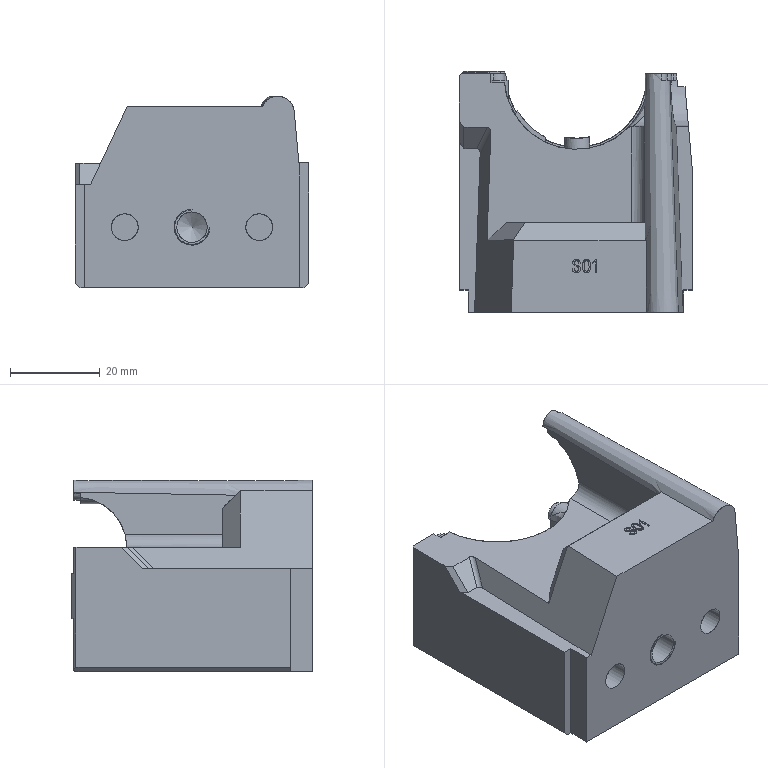NC program | PowerMill | posted with a generic post | part box 52 x 53.756 x 42.711 mm
Lines 1 to 783 of 10927:
%
O0001
N104 ( POWERMILL CB  : 2026004.0)
N105 ( POST VER      : 2026.0.0.5161)
N106 ( OPTION FILE   : FANUC)
N107 ( OUTPUT WORKPLANE : 2)
N108 (  )
N109 ( TOOL LIST )
N110 (------------------------------------)
N111 ( NO. | ID     | DIA.| TIP RAD|LENGTH)
N112 (------------------------------------)
N113 (    1|R3_1_1_1| 6.0 |  3.0   |109.48)
N114 (------------------------------------)
N115 (  )
N116 ( NUMBER OF TOOLPATHS: 2.0 )
N117 ( ESTIMATED PROGRAM DURATION: 0 HOURS 1 MIN 5 SEC)
N118 (  )
N119 G00 G21 G80 G40 G17
N120 G90
N121 G54
N122 G53 Z0.0
N123 (---------------)
N124 ( START TOOLPATH : 09中光-R3-平行-已选面 )
N125 (---------------)
N126 ( TOOL NO.    :1 )
N127 ( TOOL TYPE   : BALLNOSED)
N128 ( TOOL ID     : R3_1_1_1)
N129 ( TOOL DIA    : 6.0 LENGTH 109.48)
N130 T1
N131 M6
N132 S5500 M03
N133 G00 G90 X10.1509 Y13.0999
N134 G43 Z75.756 H1
N135
N136 G05 P10000 R8
N137 Z46.1775
N138 G01 Z43.1775 F2400.0
N139 X9.8219 Y12.7709 Z42.643 F4000.0
N140 X9.7601 Y12.7091 Z42.5428
N141 X9.7378 Y12.6936 Z42.5082
N142 X9.7126 Y12.6885 Z42.4726
N143 X9.6347 Y12.6893 Z42.3666
N144 X9.6137 Y12.7039 Z42.3403
N145 X9.6039 Y12.7473 Z42.3337
N146 X9.615 Y12.7761 Z42.3535
N147 X10.0693 Y13.2304 Z43.0441
N148 X10.3226 Y13.4837 Z43.4582
N149 X10.4866 Y13.6477 Z43.7076
N150 X10.5177 Y13.6788 Z43.7548
N151 X10.5392 Y13.7133 Z43.7877
N152 X10.5506 Y13.7612 Z43.8053
N153 X10.5572 Y13.8242 Z43.816
N154 X10.5535 Y13.8633 Z43.8107
N155 X10.5331 Y13.8905 Z43.7799
N156 X10.5116 Y13.8848 Z43.7471
N157 X10.3132 Y13.6865 Z43.4429
N158 X9.9632 Y13.3364 Z42.8782
N159 X9.4112 Y12.7844 Z42.0845
N160 X9.3531 Y12.7263 Z42.001
N161 X9.329 Y12.7098 Z41.9681
N162 X9.3018 Y12.7048 Z41.9339
N163 X9.2282 Y12.707 Z41.8449
N164 X9.2061 Y12.7217 Z41.82
N165 X9.1963 Y12.7642 Z41.8133
N166 X9.2081 Y12.7935 Z41.8313
N167 X9.6577 Y13.2431 Z42.4319
N168 X9.9859 Y13.5713 Z42.9114
N169 X10.3787 Y13.9641 Z43.5499
N170 X10.5156 Y14.101 Z43.7453
N171 X10.5378 Y14.1231 Z43.777
N172 X10.56 Y14.1619 Z43.8089
N173 X10.568 Y14.2149 Z43.8207
N174 X10.5678 Y14.259 Z43.8209
N175 X10.5601 Y14.297 Z43.8102
N176 X10.5376 Y14.3199 Z43.778
N177 X10.5151 Y14.3126 Z43.7455
N178 X10.3659 Y14.1634 Z43.5291
N179 X9.9776 Y13.7751 Z42.8993
N180 X9.6552 Y13.4527 Z42.4286
N181 X9.4 Y13.1975 Z42.0938
N182 X9.0072 Y12.8047 Z41.5949
N183 X8.9517 Y12.7492 Z41.5245
N184 X8.926 Y12.7317 Z41.4931
N185 X8.8968 Y12.7265 Z41.4603
N186 X8.8264 Y12.7296 Z41.3833
N187 X8.8035 Y12.7443 Z41.3599
N188 X8.7935 Y12.7859 Z41.3534
N189 X8.8057 Y12.8153 Z41.3699
N190 X9.322 Y13.3317 Z41.9916
N191 X9.6928 Y13.7024 Z42.4831
N192 X10.042 Y14.0516 Z42.9994
N193 X10.4706 Y14.4803 Z43.6898
N194 X10.5147 Y14.5243 Z43.7459
N195 X10.5396 Y14.5492 Z43.7776
N196 X10.562 Y14.5875 Z43.8068
N197 X10.5695 Y14.6388 Z43.8182
N198 X10.5689 Y14.6829 Z43.8192
N199 X10.5607 Y14.7209 Z43.8093
N200 X10.5376 Y14.7439 Z43.7777
N201 X10.5149 Y14.7367 Z43.7454
N202 X10.364 Y14.5858 Z43.526
N203 X9.9783 Y14.2001 Z42.9003
N204 X9.6517 Y13.8735 Z42.424
N205 X9.3429 Y13.5646 Z42.0189
N206 X8.9741 Y13.1959 Z41.5757
N207 X8.6042 Y12.8259 Z41.1544
N208 X8.5461 Y12.7679 Z41.0882
N209 X8.5193 Y12.7492 Z41.0588
N210 X8.489 Y12.7428 Z41.0276
N211 X8.4151 Y12.7426 Z40.9537
N212 X8.3912 Y12.7562 Z40.931
N213 X8.3805 Y12.7972 Z40.9238
N214 X8.3931 Y12.827 Z40.9388
N215 X8.8948 Y13.3287 Z41.482
N216 X9.265 Y13.6989 Z41.9192
N217 X9.7006 Y14.1344 Z42.4944
N218 X9.9965 Y14.4304 Z42.9268
N219 X10.3955 Y14.8294 Z43.5767
N220 X10.5158 Y14.9497 Z43.7447
N221 X10.5384 Y14.9723 Z43.7763
N222 X10.5603 Y15.0106 Z43.8075
N223 X10.5677 Y15.0628 Z43.8195
N224 X10.567 Y15.1062 Z43.8202
N225 X10.5589 Y15.1441 Z43.8101
N226 X10.5363 Y15.1671 Z43.7782
N227 X10.514 Y15.16 Z43.7458
N228 X10.3469 Y14.9929 Z43.498
N229 X10.0228 Y14.6688 Z42.9681
N230 X9.673 Y14.319 Z42.4542
N231 X9.2368 Y13.8828 Z41.8859
N232 X8.8781 Y13.5241 Z41.4629
N233 X8.5594 Y13.2054 Z41.1234
N234 X8.1745 Y12.8205 Z40.7278
N235 X8.1125 Y12.7585 Z40.664
N236 X8.0849 Y12.7389 Z40.6367
N237 X8.0538 Y12.7309 Z40.6073
N238 X7.9746 Y12.7265 Z40.5346
N239 X7.9498 Y12.7387 Z40.5126
N240 X7.9383 Y12.7791 Z40.5047
N241 X7.951 Y12.8091 Z40.5183
N242 X8.4532 Y13.3114 Z41.0111
N243 X8.914 Y13.7722 Z41.5047
N244 X9.2658 Y14.124 Z41.9201
N245 X9.7024 Y14.5606 Z42.4972
N246 X9.9981 Y14.8562 Z42.9292
N247 X10.3995 Y15.2577 Z43.583
N248 X10.4961 Y15.3543 Z43.7173
N249 X10.5025 Y15.3607 Z43.7262
N250 X10.5261 Y15.4106 Z43.7596
N251 X10.5243 Y15.4752 Z43.7589
N252 X10.5219 Y15.4847 Z43.7559
N253 X10.4934 Y15.5314 Z43.7166
N254 X10.4558 Y15.5261 Z43.6609
N255 X10.3202 Y15.3904 Z43.4542
N256 X10.0476 Y15.1179 Z43.0085
N257 X9.6376 Y14.7079 Z42.4056
N258 X9.2961 Y14.3664 Z41.9575
N259 X8.8542 Y13.9245 Z41.4374
N260 X8.4226 Y13.4929 Z40.9817
N261 X7.7332 Y12.8035 Z40.329
N262 X7.6801 Y12.7504 Z40.2787
N263 X7.6512 Y12.7307 Z40.2523
N264 X7.6185 Y12.7243 Z40.2241
N265 X7.5496 Y12.7257 Z40.1662
N266 X7.5246 Y12.7393 Z40.1463
N267 X7.5134 Y12.7789 Z40.1399
N268 X7.526 Y12.8085 Z40.1529
N269 X7.7741 Y13.0565 Z40.3808
N270 X8.0124 Y13.2949 Z40.5876
N271 X8.5224 Y13.8048 Z41.084
N272 X8.8797 Y14.1622 Z41.4646
N273 X9.2388 Y14.5212 Z41.8882
N274 X9.6759 Y14.9583 Z42.4583
N275 X10.0244 Y15.3069 Z42.9707
N276 X10.3754 Y15.6578 Z43.5403
N277 X10.3944 Y15.7105 Z43.5716
N278 X10.3823 Y15.7707 Z43.553
N279 X10.3704 Y15.7908 Z43.5343
N280 X10.3416 Y15.8158 Z43.4883
N281 X10.3106 Y15.8052 Z43.4384
N282 X10.2967 Y15.7913 Z43.4159
N283 X9.9756 Y15.4702 Z42.8964
N284 X9.6502 Y15.1448 Z42.4221
N285 X9.3327 Y14.8272 Z42.0055
N286 X8.87 Y14.3646 Z41.4543
N287 X8.5113 Y14.0059 Z41.0723
N288 X8.0059 Y13.5005 Z40.5819
N289 X7.3235 Y12.8181 Z39.9955
N290 X7.2728 Y12.7673 Z39.9518
N291 X7.243 Y12.7472 Z39.9272
N292 X7.209 Y12.7409 Z39.9006
N293 X7.1427 Y12.743 Z39.8502
N294 X7.1171 Y12.7567 Z39.8315
N295 X7.1058 Y12.7957 Z39.8252
N296 X7.1188 Y12.8255 Z39.8368
N297 X7.6223 Y13.329 Z40.2492
N298 X8.0103 Y13.717 Z40.5857
N299 X8.5202 Y14.2269 Z41.0817
N300 X8.878 Y14.5847 Z41.4628
N301 X9.2366 Y14.9433 Z41.8856
N302 X9.6727 Y15.3793 Z42.4537
N303 X10.0226 Y15.7293 Z42.9678
N304 X10.2167 Y15.9234 Z43.2851
N305 X10.2356 Y15.9764 Z43.316
N306 X10.2232 Y16.0359 Z43.2957
N307 X10.2098 Y16.0575 Z43.2738
N308 X10.1815 Y16.0809 Z43.2274
N309 X10.1511 Y16.0699 Z43.1778
N310 X10.1356 Y16.0544 Z43.1525
N311 X10.0426 Y15.9614 Z43.0004
N312 X9.6274 Y15.5462 Z42.3921
N313 X9.2788 Y15.1976 Z41.9354
N314 X8.9034 Y14.8222 Z41.4921
N315 X8.4994 Y14.4182 Z41.0595
N316 X8.0692 Y13.988 Z40.6419
N317 X7.6151 Y13.534 Z40.243
N318 X6.8996 Y12.8184 Z39.6753
N319 X6.8394 Y12.7582 Z39.6276
N320 X6.8101 Y12.7374 Z39.6051
N321 X6.7766 Y12.7283 Z39.5808
N322 X6.6971 Y12.722 Z39.5245
N323 X6.6705 Y12.7329 Z39.5069
N324 X6.657 Y12.7708 Z39.5009
N325 X6.6691 Y12.8001 Z39.5122
N326 X6.8177 Y12.9486 Z39.6302
N327 X7.0857 Y13.2166 Z39.8236
N328 X7.6226 Y13.7536 Z40.2495
N329 X8.0832 Y14.2142 Z40.6554
N330 X8.5251 Y14.656 Z41.0869
N331 X8.9493 Y15.0802 Z41.5463
N332 X9.2425 Y15.3734 Z41.8925
N333 X9.6509 Y15.7819 Z42.423
N334 X10.0501 Y16.181 Z43.0112
N335 X10.0665 Y16.2125 Z43.034
N336 X10.0692 Y16.2601 Z43.0335
N337 X10.0563 Y16.2927 Z43.0102
N338 X10.0367 Y16.3165 Z42.9772
N339 X10.007 Y16.333 Z42.9294
N340 X9.9752 Y16.3182 Z42.8823
N341 X9.9532 Y16.2963 Z42.8513
N342 X9.6846 Y16.0277 Z42.4717
N343 X9.2581 Y15.6012 Z41.911
N344 X8.9073 Y15.2504 Z41.4967
N345 X8.4379 Y14.781 Z40.9964
N346 X7.9733 Y14.3164 Z40.5536
N347 X7.571 Y13.9141 Z40.2047
N348 X7.1647 Y13.5078 Z39.8853
N349 X6.4391 Y12.7822 Z39.3593
N350 X6.3885 Y12.7316 Z39.3226
N351 X6.358 Y12.7109 Z39.3016
N352 X6.3228 Y12.7037 Z39.2791
N353 X6.2547 Z39.2373
N354 X6.2278 Y12.7161 Z39.2217
N355 X6.215 Y12.7535 Z39.2168
N356 X6.2276 Y12.7829 Z39.2268
N357 X7.0472 Y13.6024 Z39.7945
N358 X7.5603 Y14.1155 Z40.1955
N359 X7.981 Y14.5362 Z40.5603
N360 X8.454 Y15.0092 Z41.0118
N361 X8.9459 Y15.5012 Z41.5424
N362 X9.2847 Y15.8399 Z41.9426
N363 X9.8384 Y16.3936 Z42.6673
N364 X9.8541 Y16.4267 Z42.6854
N365 X9.8495 Y16.4743 Z42.672
N366 X9.8292 Y16.49 Z42.6403
N367 X9.7522 Y16.4892 Z42.5288
N368 X9.722 Y16.4816 Z42.4866
N369 X9.6928 Y16.4601 Z42.4488
N370 X9.6216 Y16.3889 Z42.3607
N371 X9.2893 Y16.0567 Z41.9498
N372 X8.9504 Y15.7178 Z41.5476
N373 X8.4568 Y15.2241 Z41.0145
N374 X7.9823 Y14.7496 Z40.5614
N375 X7.5526 Y14.32 Z40.1888
N376 X7.0373 Y13.8047 Z39.7876
N377 X6.6215 Y13.3889 Z39.4958
N378 X6.0225 Y12.7899 Z39.1007
N379 X5.9758 Y12.7431 Z39.0699
N380 X5.9443 Y12.7221 Z39.0501
N381 X5.9078 Y12.7157 Z39.0289
N382 X5.8446 Y12.7178 Z38.9933
N383 X5.8176 Y12.731 Z38.9789
N384 X5.8051 Y12.7681 Z38.9745
N385 X5.8179 Y12.7974 Z38.9838
N386 X6.5866 Y13.5661 Z39.4713
N387 X7.0382 Y14.0176 Z39.7882
N388 X7.5848 Y14.5643 Z40.2168
N389 X7.9785 Y14.958 Z40.5581
N390 X8.4487 Y15.4282 Z41.0067
N391 X8.9328 Y15.9123 Z41.5268
N392 X9.4003 Y16.3797 Z42.0696
N393 X9.4156 Y16.4123 Z42.0855
N394 X9.4092 Y16.4579 Z42.0724
N395 X9.3873 Y16.4723 Z42.0431
N396 X9.3089 Y16.4694 Z41.9439
N397 X9.2774 Y16.461 Z41.9053
N398 X9.2474 Y16.439 Z41.871
N399 X9.1777 Y16.3693 Z41.7945
N400 X8.9219 Y16.1135 Z41.5138
N401 X8.4442 Y15.6358 Z41.0024
N402 X8.0672 Y15.2588 Z40.64
N403 X7.5426 Y14.7342 Z40.1805
N404 X7.0328 Y14.2244 Z39.7844
N405 X6.6154 Y13.807 Z39.4916
N406 X6.0326 Y13.2242 Z39.1211
N407 X5.6368 Y12.8284 Z38.8873
N408 X5.6039 Y12.7955 Z38.8679
N409 X5.5689 Y12.7743 Z38.8472
N410 X5.5296 Y12.7735 Z38.8238
N411 X5.4859 Y12.7844 Z38.7979
N412 X5.4531 Y12.8202 Z38.7806
N413 X5.4653 Y12.869 Z38.7919
N414 X5.5248 Y12.9286 Z38.8332
N415 X6.0857 Y13.4895 Z39.1544
N416 X6.5171 Y13.9209 Z39.4253
N417 X7.0287 Y14.4325 Z39.7816
N418 X7.5338 Y14.9375 Z40.1736
N419 X8.0473 Y15.451 Z40.6209
N420 X8.4315 Y15.8352 Z40.9902
N421 X8.9538 Y16.3575 Z41.5307
N422 X8.9686 Y16.3896 Z41.5447
N423 X8.9605 Y16.4332 Z41.5325
N424 X8.9373 Y16.4468 Z41.5057
N425 X8.8593 Y16.4431 Z41.4193
N426 X8.8268 Y16.4345 Z41.3843
N427 X8.7966 Y16.4125 Z41.3533
N428 X8.7298 Y16.3457 Z41.2871
N429 X8.4233 Y16.0391 Z40.983
N430 X8.0405 Y15.6563 Z40.6143
N431 X7.5154 Y15.1313 Z40.1593
N432 X7.0819 Y14.6978 Z39.8207
N433 X6.6125 Y14.2284 Z39.4895
N434 X6.1132 Y13.7291 Z39.1717
N435 X5.409 Y13.0249 Z38.7721
N436 X5.3511 Y12.9669 Z38.7311
N437 X5.3504 Y12.9663 Z38.7306
N438 X5.305 Y12.9539 Z38.7018
N439 X5.2671 Y12.989 Z38.6823
N440 X5.2592 Y13.0074 Z38.6794
N441 X5.2532 Y13.0591 Z38.6793
N442 X5.2757 Y13.1037 Z38.6935
N443 X5.2896 Y13.1176 Z38.7014
N444 X6.1172 Y13.9452 Z39.1742
N445 X6.5385 Y14.3665 Z39.4387
N446 X7.0755 Y14.9035 Z39.8157
N447 X7.5073 Y15.3353 Z40.1529
N448 X7.9886 Y15.8166 Z40.5669
N449 X8.5106 Y16.3386 Z41.0565
N450 X8.5254 Y16.3703 Z41.0692
N451 X8.5171 Y16.4128 Z41.058
N452 X8.4934 Y16.4271 Z41.0331
N453 X8.4228 Y16.4276 Z40.9621
N454 X8.389 Y16.4201 Z40.929
N455 X8.3579 Y16.398 Z40.9
N456 X8.2987 Y16.3388 Z40.8468
N457 X8.0019 Y16.0421 Z40.5799
N458 X7.5564 Y15.5965 Z40.1921
N459 X7.0174 Y15.0576 Z39.7737
N460 X6.5738 Y14.614 Z39.4624
N461 X6.0921 Y14.1322 Z39.1584
N462 X5.4483 Y13.4884 Z38.7945
N463 X5.2407 Y13.2808 Z38.6665
N464 X5.196 Y13.2723 Z38.6382
N465 X5.1695 Y13.3154 Z38.6204
N466 X5.1663 Y13.3631 Z38.6173
N467 X5.1726 Y13.4102 Z38.6207
N468 X5.1962 Y13.4485 Z38.6359
N469 X5.2265 Y13.4788 Z38.6558
N470 X5.3734 Y13.6257 Z38.7521
N471 X6.0778 Y14.33 Z39.1494
N472 X6.549 Y14.8013 Z39.4453
N473 X7.1199 Y15.3722 Z39.8504
N474 X7.5246 Y15.7769 Z40.1665
N475 X8.0963 Y16.3486 Z40.6516
N476 X8.1116 Y16.3804 Z40.6629
N477 X8.1039 Y16.4224 Z40.6516
N478 X8.0801 Y16.4375 Z40.6275
N479 X8.0161 Y16.4409 Z40.5666
N480 X7.9799 Y16.4341 Z40.5337
N481 X7.9462 Y16.4106 Z40.5064
N482 X7.8926 Y16.357 Z40.4657
N483 X7.7739 Y16.2383 Z40.3759
N484 X7.5081 Y15.9725 Z40.1536
N485 X7.0637 Y15.5281 Z39.8064
N486 X6.5333 Y14.9977 Z39.4354
N487 X6.1127 Y14.5771 Z39.1713
N488 X5.2862 Y13.7506 Z38.6993
N489 X5.2169 Y13.6813 Z38.6504
N490 X5.2164 Y13.6808 Z38.65
N491 X5.1728 Y13.6739 Z38.6209
N492 X5.1473 Y13.7178 Z38.6059
N493 X5.1448 Y13.7696 Z38.6064
N494 X5.1514 Y13.8144 Z38.6118
N495 X5.1744 Y13.851 Z38.6262
N496 X5.2087 Y13.8852 Z38.6469
N497 X5.5126 Y14.1891 Z38.8304
N498 X6.0425 Y14.7191 Z39.1273
N499 X6.6364 Y15.313 Z39.5063
N500 X7.1258 Y15.8024 Z39.855
N501 X7.6854 Y16.362 Z40.287
N502 X7.7006 Y16.3939 Z40.2969
N503 X7.6914 Y16.435 Z40.2847
N504 X7.6663 Y16.4481 Z40.2614
N505 X7.594 Y16.4458 Z40.1984
N506 X7.5575 Y16.4366 Z40.168
N507 X7.5237 Y16.4124 Z40.1431
N508 X7.4642 Y16.3528 Z40.1023
N509 X7.3183 Y16.2069 Z40.0024
N510 X7.0813 Y15.9699 Z39.8202
N511 X6.5233 Y15.412 Z39.4292
N512 X6.0623 Y14.9509 Z39.1397
N513 X5.4275 Y14.3162 Z38.7829
N514 X5.2079 Y14.0966 Z38.6453
N515 X5.1804 Y14.0849 Z38.6278
N516 X5.1497 Y14.1017 Z38.6079
N517 X5.1396 Y14.1342 Z38.601
N518 X5.1399 Y14.1913 Z38.6004
N519 X5.1485 Y14.2363 Z38.6055
N520 X5.1721 Y14.2729 Z38.6206
N521 X5.2086 Y14.3094 Z38.6443
N522 X5.3871 Y14.4879 Z38.7601
N523 X6.0919 Y15.1927 Z39.1583
N524 X6.5735 Y15.6743 Z39.4622
N525 X7.2426 Y16.3434 Z39.9293
N526 X7.2574 Y16.3749 Z39.9382
N527 X7.2473 Y16.4149 Z39.927
N528 X7.2214 Y16.4277 Z39.9058
N529 X7.1507 Y16.4259 Z39.8507
N530 X7.1138 Y16.417 Z39.8232
N531 X7.0803 Y16.3933 Z39.8005
N532 X7.0235 Y16.3364 Z39.7644
N533 X6.8295 Y16.1425 Z39.6412
N534 X6.6431 Y15.956 Z39.511
N535 X6.0498 Y15.3627 Z39.1319
N536 X5.3458 Y14.6587 Z38.7358
N537 X5.2088 Y14.5218 Z38.6439
N538 X5.1815 Y14.5103 Z38.6256
N539 X5.1512 Y14.5274 Z38.6052
N540 X5.1411 Y14.5601 Z38.5984
N541 Y14.6164
N542 X5.1494 Y14.6614 Z38.604
N543 X5.1729 Y14.698 Z38.6198
N544 X5.2089 Y14.7339 Z38.6439
N545 X5.3459 Y14.871 Z38.7359
N546 X6.05 Y15.575 Z39.132
N547 X6.8271 Y16.3522 Z39.6255
N548 X6.8421 Y16.3834 Z39.6337
N549 X6.8331 Y16.4231 Z39.6238
N550 X6.8076 Y16.4382 Z39.6042
N551 X6.7496 Y16.4431 Z39.5621
N552 X6.7114 Y16.4372 Z39.5355
N553 X6.6768 Y16.414 Z39.5137
N554 X6.6306 Y16.3678 Z39.4865
N555 X6.381 Y16.1182 Z39.3397
N556 X6.0588 Y15.796 Z39.1375
N557 X5.3537 Y15.0909 Z38.7405
N558 X5.2089 Y14.9461 Z38.644
N559 X5.1816 Y14.9346 Z38.6257
N560 X5.1513 Y14.9517 Z38.6052
N561 X5.1412 Y14.9843 Z38.5983
N562 X5.1413 Y15.0407 Z38.598
N563 X5.1498 Y15.086 Z38.6036
N564 X5.1733 Y15.1226 Z38.6196
N565 X5.2089 Y15.1582 Z38.644
N566 X5.3213 Y15.2707 Z38.7211
N567 X6.0214 Y15.9707 Z39.1146
N568 X6.3273 Y16.2767 Z39.2993
N569 X6.4346 Y16.3839 Z39.3543
N570 X6.4349 Y16.3842 Z39.3544
N571 X6.4496 Y16.4154 Z39.3603
N572 X6.4384 Y16.4539 Z39.3498
N573 X6.411 Y16.4664 Z39.3319
N574 X6.3433 Y16.4655 Z39.2907
N575 X6.3058 Y16.4571 Z39.2683
N576 X6.2727 Y16.4342 Z39.2494
N577 X6.2202 Y16.3817 Z39.2203
N578 X5.3353 Y15.4967 Z38.7295
N579 X5.2157 Y15.3771 Z38.6485
N580 X5.1885 Y15.3659 Z38.63
N581 X5.1585 Y15.384 Z38.6096
N582 X5.1496 Y15.417 Z38.6035
N583 X5.152 Y15.4785 Z38.605
N584 X5.1616 Y15.5229 Z38.6115
N585 X5.1851 Y15.5587 Z38.6278
N586 X5.224 Y15.5976 Z38.6548
N587 X5.3041 Y15.6776 Z38.7104
N588 X5.8646 Y16.2382 Z39.0229
N589 X6.0005 Y16.3741 Z39.0873
N590 X6.0151 Y16.4052 Z39.0925
N591 X6.0033 Y16.4433 Z39.0819
N592 X5.9755 Y16.4551 Z39.0647
N593 X5.9062 Y16.4527 Z39.0252
N594 X5.8679 Y16.4435 Z39.0041
N595 X5.8341 Y16.4198 Z38.9872
N596 X5.7806 Y16.3663 Z38.9621
N597 X5.599 Y16.1848 Z38.877
N598 X5.3203 Y15.906 Z38.7204
N599 X5.2336 Y15.8193 Z38.661
N600 X5.2335 Y15.8192 Z38.6609
N601 X5.2063 Y15.8092 Z38.6422
N602 X5.1776 Y15.8318 Z38.6225
N603 X5.1742 Y15.866 Z38.6201
N604 X5.1961 Y15.9608 Z38.635
N605 X5.2109 Y16.0002 Z38.645
N606 X5.2347 Y16.0326 Z38.661
N607 X5.2977 Y16.0955 Z38.7033
N608 X5.3422 Y16.1401 Z38.7332
N609 X5.5074 Y16.3053 Z38.8145
N610 G00 Z44.1411
N611 G01 X1.4635 Y20.1103 F10000.0
N612 G00 Z42.0335
N613 G01 Z39.0335 F2400.0
N614 X0.9312 Y19.578 Z38.9699 F4000.0
N615 X0.7744 Y19.4212 Z38.9512
N616 X0.7457 Y19.3963 Z38.9482
N617 X0.7136 Y19.3759 Z38.9457
N618 X0.5179 Y19.2707 Z38.9325
N619 X0.4858 Y19.2687 Z38.9316
N620 X0.4614 Y19.3013 Z38.9336
N621 X0.4725 Y19.3313 Z38.9362
N622 X1.3671 Y20.2259 Z39.0294
N623 X1.9391 Y20.798 Z39.1015
N624 X2.0435 Y20.9024 Z39.1147
N625 X2.0678 Y20.9323 Z39.1179
N626 X2.0854 Y20.9665 Z39.1205
N627 X2.1394 Y21.1043 Z39.1293
N628 X2.138 Y21.1361 Z39.1298
N629 X2.1051 Y21.1579 Z39.1267
N630 X2.0756 Y21.1466 Z39.1232
N631 X1.5199 Y20.5909 Z39.0504
N632 X0.8499 Y19.9209 Z38.9726
N633 X0.1691 Y19.2401 Z38.9229
N634 X0.1158 Y19.1868 Z38.919
N635 X0.0827 Y19.1635 Z38.9173
N636 X0.0437 Y19.1528 Z38.9163
N637 X-0.0315 Y19.1456 Z38.9154
N638 X-0.0619 Y19.1545 Z38.9158
N639 X-0.078 Y19.1885 Z38.9182
N640 X-0.0656 Y19.2175 Z38.9204
N641 X0.1331 Y19.4162 Z38.9359
N642 X0.8186 Y20.1018 Z38.9688
N643 X1.4293 Y20.7124 Z39.0363
N644 X1.9821 Y21.2653 Z39.1179
N645 X2.1413 Y21.4244 Z39.1348
N646 X2.201 Y21.4841 Z39.1412
N647 X2.2244 Y21.5165 Z39.1438
N648 X2.2365 Y21.5546 Z39.1454
N649 X2.2491 Y21.6383 Z39.1477
N650 X2.2416 Y21.669 Z39.1473
N651 X2.2079 Y21.6862 Z39.1444
N652 X2.1788 Y21.6741 Z39.1414
N653 X2.0 Y21.4953 Z39.1223
N654 X1.3967 Y20.892 Z39.0288
N655 X0.9107 Y20.4059 Z38.9755
N656 X0.4555 Y19.9507 Z38.946
N657 X0.0001 Y19.4953 Z38.9354
N658 X-0.2814 Y19.2139 Z38.9228
N659 X-0.3269 Y19.1684 Z38.9208
N660 X-0.3611 Y19.1453 Z38.9201
N661 X-0.4015 Y19.1366 Z38.9206
N662 X-0.466 Y19.1354 Z38.9224
N663 X-0.5069 Y19.1619 Z38.9246
N664 X-0.4976 Y19.2098 Z38.9263
N665 X0.2904 Y19.9978 Z38.9356
N666 X0.9334 Y20.6408 Z38.9761
N667 X1.4116 Y21.119 Z39.0288
N668 X2.0149 Y21.7223 Z39.1248
N669 X2.2046 Y21.912 Z39.1449
N670 X2.2576 Y21.965 Z39.1505
N671 X2.2808 Y21.9981 Z39.153
N672 X2.2915 Y22.0372 Z39.1542
N673 X2.2986 Y22.112 Z39.1552
N674 X2.2896 Y22.1424 Z39.1543
N675 X2.2557 Y22.1586 Z39.1505
N676 X2.2267 Y22.1462 Z39.1472
N677 X1.9857 Y21.9053 Z39.1197
N678 X1.3814 Y21.301 Z39.0231
N679 X0.9611 Y20.8806 Z38.9773
N680 X0.4052 Y20.3247 Z38.9394
N681 X-0.1429 Y19.7766 Z38.9309
N682 X-0.5982 Y19.3213 Z38.939
N683 X-0.6733 Y19.2463 Z38.9317
N684 X-0.6957 Y19.2238 Z38.9295
N685 X-0.7359 Y19.2014 Z38.9277
N686 X-0.782 Y19.2034 Z38.9288
N687 X-0.8122 Y19.2135 Z38.9306
N688 X-0.8463 Y19.2507 Z38.9351
N689 X-0.8325 Y19.2992 Z38.9394
N690 X-0.724 Y19.4077 Z38.9469
N691 X-0.1169 Y20.0148 Z38.9292
N692 X0.368 Y20.4996 Z38.9354
N693 X0.8466 Y20.9783 Z38.963
N694 X1.4527 Y21.5844 Z39.0309
N695 X1.9423 Y22.0739 Z39.1114
N696 X2.2088 Y22.3405 Z39.1445
N697 X2.2444 Y22.376 Z39.1489
N698 X2.2672 Y22.4123 Z39.1515
N699 X2.2724 Y22.4549 Z39.1513
N700 X2.2673 Y22.5051 Z39.1494
N701 X2.2372 Y22.5439 Z39.1444
N702 X2.1893 Y22.5331 Z39.1381
N703 X1.9563 Y22.3001 Z39.1117
N704 X1.4752 Y21.819 Z39.0323
N705 X0.9506 Y21.2944 Z38.9719
N706 X0.3049 Y20.6487 Z38.9301
N707 X-0.2022 Y20.1416 Z38.9268
N708 X-0.8511 Y19.4927 Z38.9555
N709 X-0.9767 Y19.3671 Z38.9496
N710 X-0.9916 Y19.3522 Z38.9489
N711 X-1.0355 Y19.3299
N712 X-1.0839 Y19.3377 Z38.9518
N713 X-1.1025 Y19.3473 Z38.9535
N714 X-1.1329 Y19.3897 Z38.959
N715 X-1.1166 Y19.4393 Z38.9632
N716 X-1.0203 Y19.5356 Z38.9686
N717 X-0.4133 Y20.1426 Z38.9329
N718 X0.1343 Y20.6902 Z38.9271
N719 X0.3844 Y20.9403 Z38.9324
N720 X0.9709 Y21.5268 Z38.9719
N721 X1.4865 Y22.0424 Z39.032
N722 X1.9669 Y22.5228 Z39.1112
N723 X2.1694 Y22.7253 Z39.1308
N724 X2.2004 Y22.7563 Z39.1338
N725 X2.2231 Y22.7937 Z39.1355
N726 X2.2262 Y22.8374 Z39.1345
N727 X2.2187 Y22.8808 Z39.1321
N728 X2.1863 Y22.9181 Z39.127
N729 X2.1383 Y22.9064 Z39.122
N730 X1.9672 Y22.7353 Z39.1086
N731 X1.4787 Y22.2468 Z39.0287
N732 X0.8726 Y21.6407 Z38.9589
N733 X0.4174 Y21.1855 Z38.9325
N734 X-0.1364 Y20.6317 Z38.9235
N735 X-0.6828 Y20.0852 Z38.943
N736 X-1.1378 Y19.6303 Z38.9799
N737 X-1.2563 Y19.5118 Z38.9753
N738 X-1.271 Y19.4971 Z38.9748
N739 X-1.3149 Y19.4748 Z38.975
N740 X-1.3634 Y19.4827 Z38.9783
N741 X-1.3819 Y19.4923 Z38.9801
N742 X-1.4122 Y19.5347 Z38.9851
N743 X-1.3958 Y19.5844 Z38.9878
N744 X-1.2427 Y19.7375 Z38.9898
N745 X-0.6365 Y20.3437 Z38.9391
N746 X-0.1458 Y20.8344 Z38.9216
N747 X0.3816 Y21.3618 Z38.9276
N748 X0.9434 Y21.9236 Z38.9641
N749 X1.4187 Y22.3989 Z39.0179
N750 X1.9424 Y22.9226 Z39.1018
N751 X2.1015 Y23.0817 Z39.1123
N752 X2.1266 Y23.1068 Z39.1139
N753 X2.1492 Y23.1461 Z39.1147
N754 X2.1489 Y23.1913 Z39.1126
N755 X2.1393 Y23.2257 Z39.11
N756 X2.1037 Y23.2608 Z39.1054
N757 X2.0553 Y23.2477 Z39.1026
N758 X1.9755 Y23.1678 Z39.1013
N759 X1.5599 Y22.7522 Z39.0372
N760 X0.9215 Y22.1138 Z38.9597
N761 X0.3145 Y21.5068 Z38.9228
N762 X-0.1408 Y21.0515 Z38.9196
N763 X-0.6861 Y20.5062 Z38.9395
N764 X-1.3434 Y19.849 Z38.999
N765 X-1.5272 Y19.6651 Z39.0015
N766 X-1.5798 Y19.6439 Z39.0044
N767 X-1.6312 Y19.6672 Z39.0102
N768 X-1.6334 Y19.6696 Z39.0106
N769 X-1.6529 Y19.7221 Z39.0156
N770 X-1.6307 Y19.7738 Z39.017
N771 X-1.6284 Y19.776
N772 X-1.4456 Y19.9588 Z39.0127
N773 X-0.9488 Y20.4557 Z38.9585
N774 X-0.4071 Y20.9974 Z38.9252
N775 X0.038 Y21.4424 Z38.9191
N776 X0.3416 Y21.746 Z38.9213
N777 X1.0088 Y22.4132 Z38.9671
N778 X1.5486 Y22.953 Z39.0334
N779 X1.9593 Y23.3637 Z39.0931
N780 X2.0077 Y23.4121 Z39.0926
N781 X2.0286 Y23.4331 Z39.0924
N782 X2.051 Y23.474 Z39.0916
N783 X2.0477 Y23.5204 Z39.0902
N784 X2.0375 Y23.5478 Z39.0892
N785 X1.9991 Y23.5812 Z39.0855
N786 X1.9504 Y23.5669 Z39.0808
N787 X1.7185 Y23.3351 Z39.0581
N788 X1.5672 Y23.1837 Z39.0342
N789 X0.9197 Y22.5363 Z38.9557
N790 X0.464 Y22.0805 Z38.9264
N791 X-0.2135 Y21.4031 Z38.9144
N792 X-0.7524 Y20.8642 Z38.9387
N793 X-1.2427 Y20.3739 Z38.9847
N794 X-1.545 Y20.0716 Z39.0258
N795 X-1.7296 Y19.887 Z39.0322
N796 X-1.7818 Y19.8663 Z39.0358
N797 X-1.8322 Y19.8904 Z39.0418
N798 X-1.8355 Y19.8943 Z39.0423
N799 X-1.8537 Y19.9464 Z39.0468
N800 X-1.8315 Y19.9972 Z39.0472
N801 X-1.828 Y20.0008 Z39.0471
N802 X-1.6438 Y20.1849 Z39.0387
N803 X-1.1907 Y20.638 Z38.9779
N804 X-0.7696 Y21.0591 Z38.9376
N805 X-0.2341 Y21.5946 Z38.9127
N806 X0.4424 Y22.2711 Z38.9227
N807 X0.9671 Y22.7959 Z38.9584
N808 X1.8866 Y23.7153 Z39.0693
N809 X1.8978 Y23.7265 Z39.0706
N810 X1.9204 Y23.7726 Z39.0715
N811 X1.91 Y23.8226 Z39.0656
N812 X1.9014 Y23.8369 Z39.0628
N813 X1.8571 Y23.8653 Z39.0541
N814 X1.8068 Y23.8477 Z39.0505
N815 X1.7298 Y23.7707 Z39.0513
N816 X0.9423 Y22.9831 Z38.9541
N817 X0.3371 Y22.3779 Z38.9155
N818 X-0.1909 Y21.8499 Z38.9104
N819 X-0.7238 Y21.3171 Z38.9337
N820 X-1.244 Y20.7969 Z38.9811
N821 X-1.7424 Y20.2985 Z39.0513
N822 X-1.9233 Y20.1175 Z39.0615
N823 X-1.9751 Y20.0975 Z39.0659
N824 X-2.0245 Y20.1224 Z39.072
N825 X-2.0289 Y20.1277 Z39.0727
N826 X-2.0458 Y20.1795 Z39.0766
N827 X-2.0236 Y20.2294 Z39.0761
N828 X-2.0187 Y20.2343 Z39.0758
N829 X-1.8367 Y20.4163 Z39.0634
N830 X-1.3281 Y20.9248 Z38.9876
N831 X-0.7237 Y21.5293 Z38.9319
N832 X-0.2471 Y22.0059 Z38.9094
N833 X0.3567 Y22.6097 Z38.9144
N834 X1.0216 Y23.2746 Z38.9602
N835 X1.7239 Y23.9769 Z39.0407
N836 X1.7334 Y23.9864 Z39.0418
N837 X1.756 Y24.0334 Z39.0424
N838 X1.7441 Y24.0838 Z39.0363
N839 X1.7361 Y24.096 Z39.0338
N840 X1.6907 Y24.1235 Z39.0257
N841 X1.6401 Y24.1053 Z39.0235
N842 X1.6051 Y24.0703 Z39.0251
N843 X1.1078 Y23.573 Z38.9674
N844 X0.4323 Y22.8974 Z38.9161
N845 X-0.1571 Y22.308 Z38.9065
N846 X-0.7907 Y21.6745 Z38.933
N847 X-1.2843 Y21.1809 Z38.9813
N848 X-1.9307 Y20.5344 Z39.0783
N849 X-2.1141 Y20.351 Z39.091
N850 X-2.165 Y20.3323 Z39.0959
N851 X-2.2121 Y20.359 Z39.1021
N852 X-2.2187 Y20.3683 Z39.1032
N853 X-2.2326 Y20.4191 Z39.1068
N854 X-2.2103 Y20.4669 Z39.1063
N855 X-2.2023 Y20.475 Z39.1058
N856 X-2.0251 Y20.6521 Z39.094
N857 X-1.2695 Y21.4078 Z38.978
N858 X-0.823 Y21.8542 Z38.9335
N859 X-0.1874 Y22.4898 Z38.9048
N860 X0.4107 Y23.088 Z38.913
N861 X1.0815 Y23.7588 Z38.9625
N862 X1.556 Y24.2332 Z39.0105
N863 X1.5655 Y24.2427 Z39.0115
N864 X1.5881 Y24.2899 Z39.0117
N865 X1.576 Y24.3405 Z39.0051
N866 X1.5683 Y24.3522 Z39.0027
N867 X1.5226 Y24.3797 Z38.9935
N868 X1.4719 Y24.3613 Z38.9893
N869 X1.331 Y24.2204 Z38.9888
N870 X1.1026 Y23.992 Z38.9627
N871 X0.4247 Y23.3141 Z38.9118
N872 X-0.1778 Y22.7115 Z38.9028
N873 X-0.8141 Y22.0752 Z38.9309
N874 X-1.2591 Y21.6303 Z38.9751
N875 X-1.8176 Y21.0718 Z39.055
N876 X-2.1197 Y20.7697 Z39.1097
N877 X-2.2843 Y20.6051 Z39.1199
N878 X-2.3337 Y20.5891 Z39.1243
N879 X-2.3755 Y20.62 Z39.1297
N880 X-2.3853 Y20.6398 Z39.1315